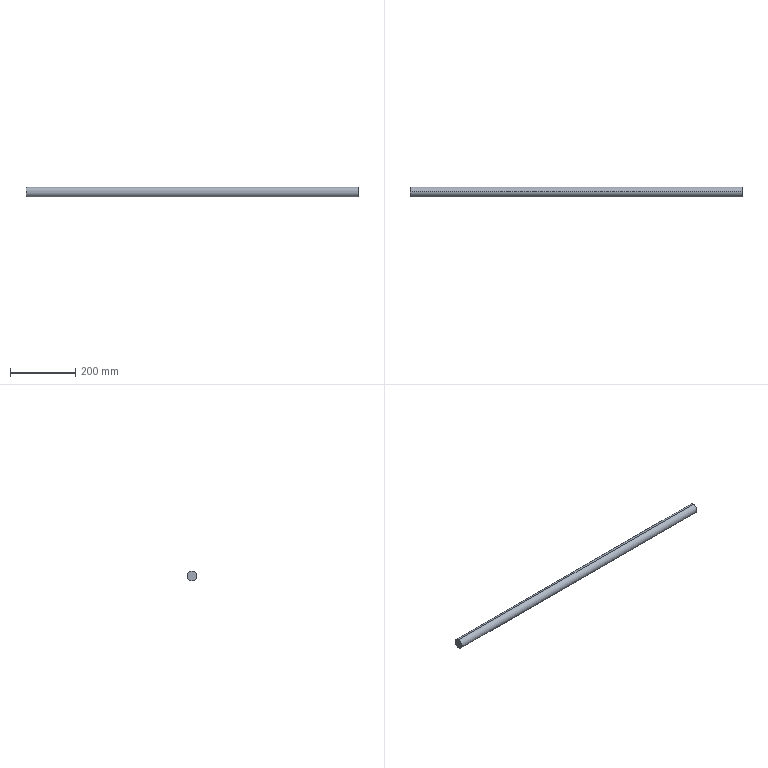Part | SolidWorks | features ICE 3, WeldMemberFeat 1, WeldmentFeature 1 | 1 solid | 4 faces | box 1022 x 30 x 30 mm | volume 722056 mm3 | cylinder 2 | plane 2 | commonest cylinder face diameters 30 x2
STEP:
#1=CARTESIAN_POINT('',(1021.5,0.,-15.));
#2=VERTEX_POINT('',#1);
#3=CARTESIAN_POINT('',(1021.5,0.,15.));
#4=VERTEX_POINT('',#3);
#5=CARTESIAN_POINT('',(1021.5,0.,0.));
#6=DIRECTION('',(1.,0.,0.));
#7=DIRECTION('',(0.,0.,-1.));
#8=AXIS2_PLACEMENT_3D('',#5,#6,#7);
#9=CIRCLE('',#8,15.);
#10=EDGE_CURVE('',#2,#4,#9,.T.);
#11=ORIENTED_EDGE('',*,*,#10,.F.);
#12=CARTESIAN_POINT('',(0.,0.,-15.));
#13=VERTEX_POINT('',#12);
#14=CARTESIAN_POINT('',(1021.5,0.,-15.));
#15=DIRECTION('',(-1.,0.,0.));
#16=VECTOR('',#15,1000.);
#17=LINE('',#14,#16);
#18=EDGE_CURVE('',#2,#13,#17,.T.);
#19=ORIENTED_EDGE('',*,*,#18,.T.);
#20=CARTESIAN_POINT('',(0.,0.,15.));
#21=VERTEX_POINT('',#20);
#22=CARTESIAN_POINT('',(0.,0.,0.));
#23=DIRECTION('',(1.,0.,0.));
#24=DIRECTION('',(0.,0.,-1.));
#25=AXIS2_PLACEMENT_3D('',#22,#23,#24);
#26=CIRCLE('',#25,15.);
#27=EDGE_CURVE('',#13,#21,#26,.T.);
#28=ORIENTED_EDGE('',*,*,#27,.T.);
#29=CARTESIAN_POINT('',(1021.5,0.,15.));
#30=DIRECTION('',(-1.,0.,0.));
#31=VECTOR('',#30,1000.);
#32=LINE('',#29,#31);
#33=EDGE_CURVE('',#4,#21,#32,.T.);
#34=ORIENTED_EDGE('',*,*,#33,.F.);
#35=EDGE_LOOP('',(#11,#19,#28,#34));
#36=FACE_OUTER_BOUND('',#35,.T.);
#37=CARTESIAN_POINT('',(1021.5,0.,0.));
#38=DIRECTION('',(-1.,0.,0.));
#39=DIRECTION('',(0.,0.,1.));
#40=AXIS2_PLACEMENT_3D('',#37,#38,#39);
#41=CYLINDRICAL_SURFACE('',#40,15.);
#42=ADVANCED_FACE('',(#36),#41,.T.);
#43=ORIENTED_EDGE('',*,*,#18,.F.);
#44=CARTESIAN_POINT('',(1021.5,0.,0.));
#45=DIRECTION('',(1.,0.,0.));
#46=DIRECTION('',(0.,0.,-1.));
#47=AXIS2_PLACEMENT_3D('',#44,#45,#46);
#48=CIRCLE('',#47,15.);
#49=EDGE_CURVE('',#4,#2,#48,.T.);
#50=ORIENTED_EDGE('',*,*,#49,.F.);
#51=ORIENTED_EDGE('',*,*,#33,.T.);
#52=CARTESIAN_POINT('',(0.,0.,0.));
#53=DIRECTION('',(1.,0.,0.));
#54=DIRECTION('',(0.,0.,-1.));
#55=AXIS2_PLACEMENT_3D('',#52,#53,#54);
#56=CIRCLE('',#55,15.);
#57=EDGE_CURVE('',#21,#13,#56,.T.);
#58=ORIENTED_EDGE('',*,*,#57,.T.);
#59=EDGE_LOOP('',(#43,#50,#51,#58));
#60=FACE_OUTER_BOUND('',#59,.T.);
#61=CARTESIAN_POINT('',(1021.5,0.,0.));
#62=DIRECTION('',(-1.,0.,0.));
#63=DIRECTION('',(0.,0.,1.));
#64=AXIS2_PLACEMENT_3D('',#61,#62,#63);
#65=CYLINDRICAL_SURFACE('',#64,15.);
#66=ADVANCED_FACE('',(#60),#65,.T.);
#67=ORIENTED_EDGE('',*,*,#49,.T.);
#68=ORIENTED_EDGE('',*,*,#10,.T.);
#69=EDGE_LOOP('',(#67,#68));
#70=FACE_OUTER_BOUND('',#69,.T.);
#71=CARTESIAN_POINT('',(1021.5,0.,0.));
#72=DIRECTION('',(1.,0.,0.));
#73=DIRECTION('',(0.,0.,-1.));
#74=AXIS2_PLACEMENT_3D('',#71,#72,#73);
#75=PLANE('',#74);
#76=ADVANCED_FACE('',(#70),#75,.T.);
#77=ORIENTED_EDGE('',*,*,#57,.F.);
#78=ORIENTED_EDGE('',*,*,#27,.F.);
#79=EDGE_LOOP('',(#77,#78));
#80=FACE_OUTER_BOUND('',#79,.T.);
#81=CARTESIAN_POINT('',(0.,0.,0.));
#82=DIRECTION('',(1.,0.,0.));
#83=DIRECTION('',(0.,0.,-1.));
#84=AXIS2_PLACEMENT_3D('',#81,#82,#83);
#85=PLANE('',#84);
#86=ADVANCED_FACE('',(#80),#85,.F.);
#87=CLOSED_SHELL('',(#42,#66,#76,#86));
#88=MANIFOLD_SOLID_BREP('',#87);
#89=CARTESIAN_POINT('',(0.,0.,0.));
#90=DIRECTION('',(0.,0.,1.));
#91=DIRECTION('',(1.,0.,0.));
#92=AXIS2_PLACEMENT_3D('',#89,#90,#91);
#93=(LENGTH_UNIT()NAMED_UNIT(*)SI_UNIT(.MILLI.,.METRE.));
#94=UNCERTAINTY_MEASURE_WITH_UNIT(LENGTH_MEASURE(0.00001),#93,'','');
#95=(NAMED_UNIT(*)PLANE_ANGLE_UNIT()SI_UNIT($,.RADIAN.));
#96=(NAMED_UNIT(*)SI_UNIT($,.STERADIAN.)SOLID_ANGLE_UNIT());
#97=(GEOMETRIC_REPRESENTATION_CONTEXT(3)GLOBAL_UNCERTAINTY_ASSIGNED_CONTEXT((#94))GLOBAL_UNIT_ASSIGNED_CONTEXT((#93,#95,#96))REPRESENTATION_CONTEXT('',''));
#98=ADVANCED_BREP_SHAPE_REPRESENTATION('',(#88,#92),#97);